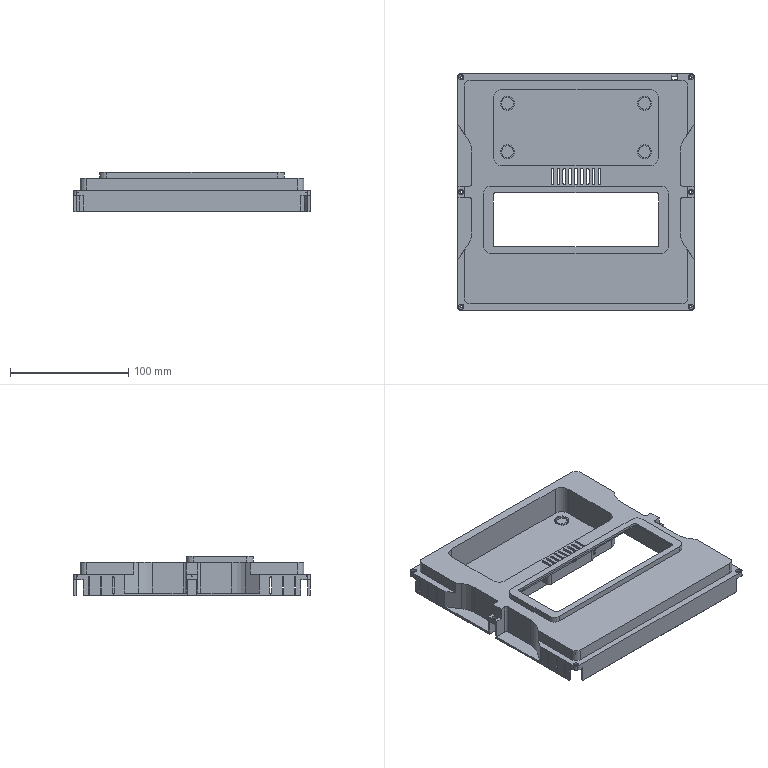Part | SolidWorks | features ICE 31, Fillet 3, Chamfer 1, Extrusion 1, LPattern 1, MirrorPattern 1, Shell 1 | 1 solid | 419 faces | box 199.7 x 199.7 x 33 mm | volume 138298 mm3 | plane 282 | cylinder 137 | commonest cylinder face diameters 1.5 x24 2 x24 4 x14 2.2 x12 4.5 x12 12 x12